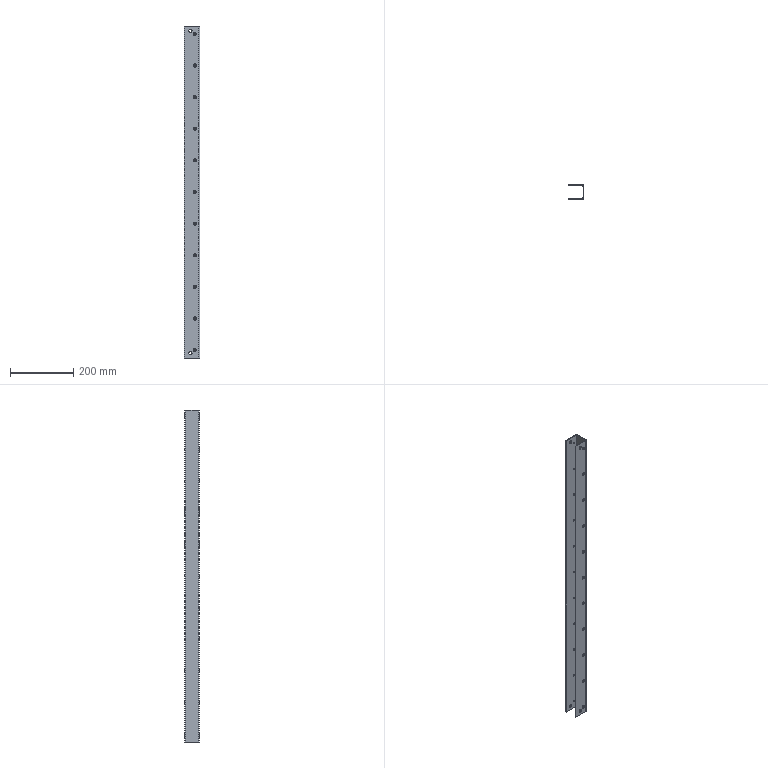Part | NX | features BREP 1 | 1 solid | 66 faces | box 50 x 45 x 1050 mm | volume 357061 mm3 | cylinder 56 | plane 10 | commonest cylinder face diameters 5.5 x22 10 x22 10.5 x8 2 x2 8 x2